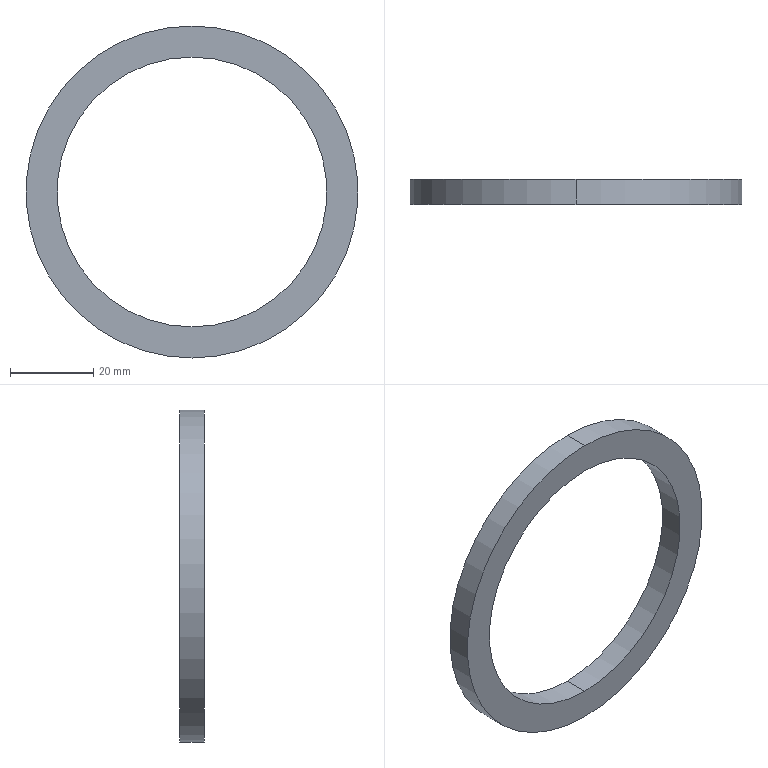Part | SolidWorks | features Extrusion 1 | 1 solid | 6 faces | box 80 x 6 x 80 mm | volume 10249 mm3 | cylinder 4 | plane 2 | commonest cylinder face diameters 65 x2 80 x2
STEP:
#1=CARTESIAN_POINT('',(0.,6.,-32.5));
#2=VERTEX_POINT('',#1);
#3=CARTESIAN_POINT('',(0.,6.,32.5));
#4=VERTEX_POINT('',#3);
#5=CARTESIAN_POINT('',(0.,6.,0.));
#6=DIRECTION('',(0.,1.,0.));
#7=DIRECTION('',(0.,0.,1.));
#8=AXIS2_PLACEMENT_3D('',#5,#6,#7);
#9=CIRCLE('',#8,32.5);
#10=EDGE_CURVE('',#2,#4,#9,.T.);
#11=ORIENTED_EDGE('',*,*,#10,.T.);
#12=CARTESIAN_POINT('',(0.,0.,32.5));
#13=VERTEX_POINT('',#12);
#14=CARTESIAN_POINT('',(0.,6.,32.5));
#15=DIRECTION('',(0.,-1.,0.));
#16=VECTOR('',#15,1000.);
#17=LINE('',#14,#16);
#18=EDGE_CURVE('',#4,#13,#17,.T.);
#19=ORIENTED_EDGE('',*,*,#18,.T.);
#20=CARTESIAN_POINT('',(0.,0.,-32.5));
#21=VERTEX_POINT('',#20);
#22=CARTESIAN_POINT('',(0.,0.,0.));
#23=DIRECTION('',(0.,1.,0.));
#24=DIRECTION('',(0.,0.,1.));
#25=AXIS2_PLACEMENT_3D('',#22,#23,#24);
#26=CIRCLE('',#25,32.5);
#27=EDGE_CURVE('',#21,#13,#26,.T.);
#28=ORIENTED_EDGE('',*,*,#27,.F.);
#29=CARTESIAN_POINT('',(0.,6.,-32.5));
#30=DIRECTION('',(0.,-1.,0.));
#31=VECTOR('',#30,1000.);
#32=LINE('',#29,#31);
#33=EDGE_CURVE('',#2,#21,#32,.T.);
#34=ORIENTED_EDGE('',*,*,#33,.F.);
#35=EDGE_LOOP('',(#11,#19,#28,#34));
#36=FACE_OUTER_BOUND('',#35,.T.);
#37=CARTESIAN_POINT('',(0.,6.,0.));
#38=DIRECTION('',(0.,-1.,0.));
#39=DIRECTION('',(0.,0.,-1.));
#40=AXIS2_PLACEMENT_3D('',#37,#38,#39);
#41=CYLINDRICAL_SURFACE('',#40,32.5);
#42=ADVANCED_FACE('',(#36),#41,.F.);
#43=CARTESIAN_POINT('',(0.,6.,40.));
#44=VERTEX_POINT('',#43);
#45=CARTESIAN_POINT('',(0.,6.,-40.));
#46=VERTEX_POINT('',#45);
#47=CARTESIAN_POINT('',(0.,6.,0.));
#48=DIRECTION('',(0.,1.,0.));
#49=DIRECTION('',(0.,0.,1.));
#50=AXIS2_PLACEMENT_3D('',#47,#48,#49);
#51=CIRCLE('',#50,40.);
#52=EDGE_CURVE('',#44,#46,#51,.T.);
#53=ORIENTED_EDGE('',*,*,#52,.F.);
#54=CARTESIAN_POINT('',(0.,0.,40.));
#55=VERTEX_POINT('',#54);
#56=CARTESIAN_POINT('',(0.,6.,40.));
#57=DIRECTION('',(0.,-1.,0.));
#58=VECTOR('',#57,1000.);
#59=LINE('',#56,#58);
#60=EDGE_CURVE('',#44,#55,#59,.T.);
#61=ORIENTED_EDGE('',*,*,#60,.T.);
#62=CARTESIAN_POINT('',(0.,0.,-40.));
#63=VERTEX_POINT('',#62);
#64=CARTESIAN_POINT('',(0.,0.,0.));
#65=DIRECTION('',(0.,1.,0.));
#66=DIRECTION('',(0.,0.,1.));
#67=AXIS2_PLACEMENT_3D('',#64,#65,#66);
#68=CIRCLE('',#67,40.);
#69=EDGE_CURVE('',#55,#63,#68,.T.);
#70=ORIENTED_EDGE('',*,*,#69,.T.);
#71=CARTESIAN_POINT('',(0.,6.,-40.));
#72=DIRECTION('',(0.,-1.,0.));
#73=VECTOR('',#72,1000.);
#74=LINE('',#71,#73);
#75=EDGE_CURVE('',#46,#63,#74,.T.);
#76=ORIENTED_EDGE('',*,*,#75,.F.);
#77=EDGE_LOOP('',(#53,#61,#70,#76));
#78=FACE_OUTER_BOUND('',#77,.T.);
#79=CARTESIAN_POINT('',(0.,6.,0.));
#80=DIRECTION('',(0.,-1.,0.));
#81=DIRECTION('',(0.,0.,-1.));
#82=AXIS2_PLACEMENT_3D('',#79,#80,#81);
#83=CYLINDRICAL_SURFACE('',#82,40.);
#84=ADVANCED_FACE('',(#78),#83,.T.);
#85=CARTESIAN_POINT('',(0.,6.,0.));
#86=DIRECTION('',(0.,1.,0.));
#87=DIRECTION('',(0.,0.,1.));
#88=AXIS2_PLACEMENT_3D('',#85,#86,#87);
#89=CIRCLE('',#88,40.);
#90=EDGE_CURVE('',#46,#44,#89,.T.);
#91=ORIENTED_EDGE('',*,*,#90,.T.);
#92=ORIENTED_EDGE('',*,*,#52,.T.);
#93=EDGE_LOOP('',(#91,#92));
#94=FACE_OUTER_BOUND('',#93,.T.);
#95=ORIENTED_EDGE('',*,*,#10,.F.);
#96=CARTESIAN_POINT('',(0.,6.,0.));
#97=DIRECTION('',(0.,1.,0.));
#98=DIRECTION('',(0.,0.,1.));
#99=AXIS2_PLACEMENT_3D('',#96,#97,#98);
#100=CIRCLE('',#99,32.5);
#101=EDGE_CURVE('',#4,#2,#100,.T.);
#102=ORIENTED_EDGE('',*,*,#101,.F.);
#103=EDGE_LOOP('',(#95,#102));
#104=FACE_BOUND('',#103,.T.);
#105=CARTESIAN_POINT('',(0.,6.,0.));
#106=DIRECTION('',(0.,1.,0.));
#107=DIRECTION('',(0.,0.,1.));
#108=AXIS2_PLACEMENT_3D('',#105,#106,#107);
#109=PLANE('',#108);
#110=ADVANCED_FACE('',(#94,#104),#109,.T.);
#111=CARTESIAN_POINT('',(0.,0.,0.));
#112=DIRECTION('',(0.,1.,0.));
#113=DIRECTION('',(0.,0.,1.));
#114=AXIS2_PLACEMENT_3D('',#111,#112,#113);
#115=CIRCLE('',#114,40.);
#116=EDGE_CURVE('',#63,#55,#115,.T.);
#117=ORIENTED_EDGE('',*,*,#116,.F.);
#118=ORIENTED_EDGE('',*,*,#69,.F.);
#119=EDGE_LOOP('',(#117,#118));
#120=FACE_OUTER_BOUND('',#119,.T.);
#121=ORIENTED_EDGE('',*,*,#27,.T.);
#122=CARTESIAN_POINT('',(0.,0.,0.));
#123=DIRECTION('',(0.,1.,0.));
#124=DIRECTION('',(0.,0.,1.));
#125=AXIS2_PLACEMENT_3D('',#122,#123,#124);
#126=CIRCLE('',#125,32.5);
#127=EDGE_CURVE('',#13,#21,#126,.T.);
#128=ORIENTED_EDGE('',*,*,#127,.T.);
#129=EDGE_LOOP('',(#121,#128));
#130=FACE_BOUND('',#129,.T.);
#131=CARTESIAN_POINT('',(0.,0.,0.));
#132=DIRECTION('',(0.,1.,0.));
#133=DIRECTION('',(0.,0.,1.));
#134=AXIS2_PLACEMENT_3D('',#131,#132,#133);
#135=PLANE('',#134);
#136=ADVANCED_FACE('',(#120,#130),#135,.F.);
#137=ORIENTED_EDGE('',*,*,#60,.F.);
#138=ORIENTED_EDGE('',*,*,#90,.F.);
#139=ORIENTED_EDGE('',*,*,#75,.T.);
#140=ORIENTED_EDGE('',*,*,#116,.T.);
#141=EDGE_LOOP('',(#137,#138,#139,#140));
#142=FACE_OUTER_BOUND('',#141,.T.);
#143=CARTESIAN_POINT('',(0.,6.,0.));
#144=DIRECTION('',(0.,-1.,0.));
#145=DIRECTION('',(0.,0.,-1.));
#146=AXIS2_PLACEMENT_3D('',#143,#144,#145);
#147=CYLINDRICAL_SURFACE('',#146,40.);
#148=ADVANCED_FACE('',(#142),#147,.T.);
#149=ORIENTED_EDGE('',*,*,#18,.F.);
#150=ORIENTED_EDGE('',*,*,#101,.T.);
#151=ORIENTED_EDGE('',*,*,#33,.T.);
#152=ORIENTED_EDGE('',*,*,#127,.F.);
#153=EDGE_LOOP('',(#149,#150,#151,#152));
#154=FACE_OUTER_BOUND('',#153,.T.);
#155=CARTESIAN_POINT('',(0.,6.,0.));
#156=DIRECTION('',(0.,-1.,0.));
#157=DIRECTION('',(0.,0.,-1.));
#158=AXIS2_PLACEMENT_3D('',#155,#156,#157);
#159=CYLINDRICAL_SURFACE('',#158,32.5);
#160=ADVANCED_FACE('',(#154),#159,.F.);
#161=CLOSED_SHELL('',(#42,#84,#110,#136,#148,#160));
#162=MANIFOLD_SOLID_BREP('',#161);
#163=CARTESIAN_POINT('',(0.,0.,0.));
#164=DIRECTION('',(0.,0.,1.));
#165=DIRECTION('',(1.,0.,0.));
#166=AXIS2_PLACEMENT_3D('',#163,#164,#165);
#167=(LENGTH_UNIT()NAMED_UNIT(*)SI_UNIT(.MILLI.,.METRE.));
#168=UNCERTAINTY_MEASURE_WITH_UNIT(LENGTH_MEASURE(0.00001),#167,'','');
#169=(NAMED_UNIT(*)PLANE_ANGLE_UNIT()SI_UNIT($,.RADIAN.));
#170=(NAMED_UNIT(*)SI_UNIT($,.STERADIAN.)SOLID_ANGLE_UNIT());
#171=(GEOMETRIC_REPRESENTATION_CONTEXT(3)GLOBAL_UNCERTAINTY_ASSIGNED_CONTEXT((#168))GLOBAL_UNIT_ASSIGNED_CONTEXT((#167,#169,#170))REPRESENTATION_CONTEXT('',''));
#172=ADVANCED_BREP_SHAPE_REPRESENTATION('',(#162,#166),#171);